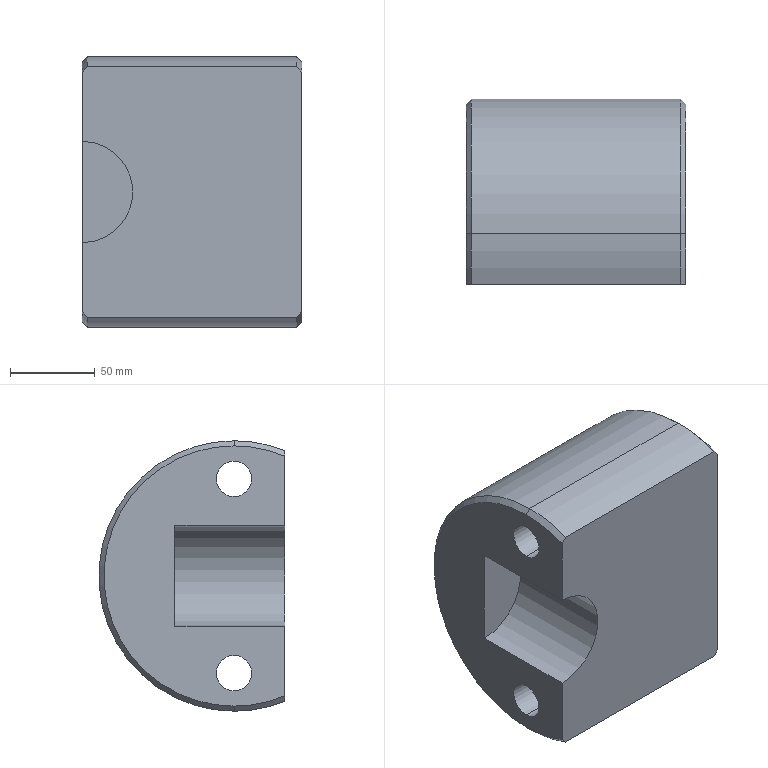Part | SolidWorks | features BaseBody 1 | 1 solid | 18 faces | box 130 x 110 x 160 mm | volume 1731219 mm3 | cylinder 8 | cone 6 | plane 4 | commonest cylinder face diameters 21 x4 160 x3 60 x1
STEP:
#1=CARTESIAN_POINT('',(240.077,193.635,-171.893));
#2=VERTEX_POINT('',#1);
#3=CARTESIAN_POINT('',(370.077,193.635,-171.893));
#4=VERTEX_POINT('',#3);
#5=CARTESIAN_POINT('',(370.077,193.635,-171.893));
#6=DIRECTION('',(1.,0.,0.));
#7=VECTOR('',#6,1000.);
#8=LINE('',#5,#7);
#9=EDGE_CURVE('',#2,#4,#8,.T.);
#10=ORIENTED_EDGE('',*,*,#9,.F.);
#11=CARTESIAN_POINT('',(240.077,193.635,-192.893));
#12=VERTEX_POINT('',#11);
#13=CARTESIAN_POINT('',(240.077,193.635,-182.393));
#14=DIRECTION('',(1.,0.,0.));
#15=DIRECTION('',(0.,0.,-1.));
#16=AXIS2_PLACEMENT_3D('',#13,#14,#15);
#17=CIRCLE('',#16,10.5);
#18=EDGE_CURVE('',#12,#2,#17,.T.);
#19=ORIENTED_EDGE('',*,*,#18,.F.);
#20=CARTESIAN_POINT('',(370.077,193.635,-192.893));
#21=VERTEX_POINT('',#20);
#22=CARTESIAN_POINT('',(370.077,193.635,-192.893));
#23=DIRECTION('',(1.,0.,0.));
#24=VECTOR('',#23,1000.);
#25=LINE('',#22,#24);
#26=EDGE_CURVE('',#12,#21,#25,.T.);
#27=ORIENTED_EDGE('',*,*,#26,.T.);
#28=CARTESIAN_POINT('',(370.077,193.635,-182.393));
#29=DIRECTION('',(1.,0.,0.));
#30=DIRECTION('',(0.,0.,-1.));
#31=AXIS2_PLACEMENT_3D('',#28,#29,#30);
#32=CIRCLE('',#31,10.5);
#33=EDGE_CURVE('',#21,#4,#32,.T.);
#34=ORIENTED_EDGE('',*,*,#33,.T.);
#35=EDGE_LOOP('',(#10,#19,#27,#34));
#36=FACE_OUTER_BOUND('',#35,.T.);
#37=CARTESIAN_POINT('',(370.077,193.635,-182.393));
#38=DIRECTION('',(1.,0.,0.));
#39=DIRECTION('',(0.,0.,-1.));
#40=AXIS2_PLACEMENT_3D('',#37,#38,#39);
#41=CYLINDRICAL_SURFACE('',#40,10.5);
#42=ADVANCED_FACE('',(#36),#41,.F.);
#43=CARTESIAN_POINT('',(240.077,193.635,-286.893));
#44=VERTEX_POINT('',#43);
#45=CARTESIAN_POINT('',(370.077,193.635,-286.893));
#46=VERTEX_POINT('',#45);
#47=CARTESIAN_POINT('',(370.077,193.635,-286.893));
#48=DIRECTION('',(1.,0.,0.));
#49=VECTOR('',#48,1000.);
#50=LINE('',#47,#49);
#51=EDGE_CURVE('',#44,#46,#50,.T.);
#52=ORIENTED_EDGE('',*,*,#51,.F.);
#53=CARTESIAN_POINT('',(240.077,193.635,-307.893));
#54=VERTEX_POINT('',#53);
#55=CARTESIAN_POINT('',(240.077,193.635,-297.393));
#56=DIRECTION('',(1.,0.,0.));
#57=DIRECTION('',(0.,0.,-1.));
#58=AXIS2_PLACEMENT_3D('',#55,#56,#57);
#59=CIRCLE('',#58,10.5);
#60=EDGE_CURVE('',#54,#44,#59,.T.);
#61=ORIENTED_EDGE('',*,*,#60,.F.);
#62=CARTESIAN_POINT('',(370.077,193.635,-307.893));
#63=VERTEX_POINT('',#62);
#64=CARTESIAN_POINT('',(370.077,193.635,-307.893));
#65=DIRECTION('',(1.,0.,0.));
#66=VECTOR('',#65,1000.);
#67=LINE('',#64,#66);
#68=EDGE_CURVE('',#54,#63,#67,.T.);
#69=ORIENTED_EDGE('',*,*,#68,.T.);
#70=CARTESIAN_POINT('',(370.077,193.635,-297.393));
#71=DIRECTION('',(1.,0.,0.));
#72=DIRECTION('',(0.,0.,-1.));
#73=AXIS2_PLACEMENT_3D('',#70,#71,#72);
#74=CIRCLE('',#73,10.5);
#75=EDGE_CURVE('',#63,#46,#74,.T.);
#76=ORIENTED_EDGE('',*,*,#75,.T.);
#77=EDGE_LOOP('',(#52,#61,#69,#76));
#78=FACE_OUTER_BOUND('',#77,.T.);
#79=CARTESIAN_POINT('',(370.077,193.635,-297.393));
#80=DIRECTION('',(1.,0.,0.));
#81=DIRECTION('',(0.,0.,-1.));
#82=AXIS2_PLACEMENT_3D('',#79,#80,#81);
#83=CYLINDRICAL_SURFACE('',#82,10.5);
#84=ADVANCED_FACE('',(#78),#83,.F.);
#85=CARTESIAN_POINT('',(240.077,228.635,-269.893));
#86=VERTEX_POINT('',#85);
#87=CARTESIAN_POINT('',(240.077,228.635,-209.893));
#88=VERTEX_POINT('',#87);
#89=CARTESIAN_POINT('',(240.077,228.635,-239.893));
#90=DIRECTION('',(0.,-1.,0.));
#91=DIRECTION('',(0.,0.,-1.));
#92=AXIS2_PLACEMENT_3D('',#89,#90,#91);
#93=CIRCLE('',#92,30.);
#94=EDGE_CURVE('',#86,#88,#93,.T.);
#95=ORIENTED_EDGE('',*,*,#94,.F.);
#96=CARTESIAN_POINT('',(240.077,163.635,-269.893));
#97=VERTEX_POINT('',#96);
#98=CARTESIAN_POINT('',(240.077,228.635,-269.893));
#99=DIRECTION('',(0.,1.,0.));
#100=VECTOR('',#99,1000.);
#101=LINE('',#98,#100);
#102=EDGE_CURVE('',#97,#86,#101,.T.);
#103=ORIENTED_EDGE('',*,*,#102,.F.);
#104=CARTESIAN_POINT('',(240.077,163.635,-209.893));
#105=VERTEX_POINT('',#104);
#106=CARTESIAN_POINT('',(240.077,163.635,-239.893));
#107=DIRECTION('',(0.,-1.,0.));
#108=DIRECTION('',(0.,0.,-1.));
#109=AXIS2_PLACEMENT_3D('',#106,#107,#108);
#110=CIRCLE('',#109,30.);
#111=EDGE_CURVE('',#97,#105,#110,.T.);
#112=ORIENTED_EDGE('',*,*,#111,.T.);
#113=CARTESIAN_POINT('',(240.077,228.635,-209.893));
#114=DIRECTION('',(0.,-1.,0.));
#115=VECTOR('',#114,1000.);
#116=LINE('',#113,#115);
#117=EDGE_CURVE('',#88,#105,#116,.T.);
#118=ORIENTED_EDGE('',*,*,#117,.F.);
#119=EDGE_LOOP('',(#95,#103,#112,#118));
#120=FACE_OUTER_BOUND('',#119,.T.);
#121=CARTESIAN_POINT('',(240.077,228.635,-239.893));
#122=DIRECTION('',(0.,-1.,0.));
#123=DIRECTION('',(0.,0.,1.));
#124=AXIS2_PLACEMENT_3D('',#121,#122,#123);
#125=CYLINDRICAL_SURFACE('',#124,30.);
#126=ADVANCED_FACE('',(#120),#125,.F.);
#127=CARTESIAN_POINT('',(240.077,228.635,-239.893));
#128=DIRECTION('',(0.,0.,-1.));
#129=VECTOR('',#128,1000.);
#130=LINE('',#127,#129);
#131=EDGE_CURVE('',#88,#86,#130,.T.);
#132=ORIENTED_EDGE('',*,*,#131,.T.);
#133=ORIENTED_EDGE('',*,*,#94,.T.);
#134=EDGE_LOOP('',(#132,#133));
#135=FACE_OUTER_BOUND('',#134,.T.);
#136=CARTESIAN_POINT('',(240.077,228.635,-239.893));
#137=DIRECTION('',(0.,-1.,0.));
#138=DIRECTION('',(0.,0.,-1.));
#139=AXIS2_PLACEMENT_3D('',#136,#137,#138);
#140=PLANE('',#139);
#141=ADVANCED_FACE('',(#135),#140,.T.);
#142=CARTESIAN_POINT('',(240.077,193.635,-162.893));
#143=VERTEX_POINT('',#142);
#144=CARTESIAN_POINT('',(243.077,193.635,-159.893));
#145=VERTEX_POINT('',#144);
#146=CARTESIAN_POINT('',(243.077,193.635,-159.893));
#147=DIRECTION('',(0.7071,0.,0.7071));
#148=VECTOR('',#147,1000.);
#149=LINE('',#146,#148);
#150=EDGE_CURVE('',#143,#145,#149,.T.);
#151=ORIENTED_EDGE('',*,*,#150,.F.);
#152=CARTESIAN_POINT('',(240.077,163.635,-168.978));
#153=VERTEX_POINT('',#152);
#154=CARTESIAN_POINT('',(240.077,193.635,-239.893));
#155=DIRECTION('',(-1.,0.,0.));
#156=DIRECTION('',(0.,0.,-1.));
#157=AXIS2_PLACEMENT_3D('',#154,#155,#156);
#158=CIRCLE('',#157,77.);
#159=EDGE_CURVE('',#153,#143,#158,.T.);
#160=ORIENTED_EDGE('',*,*,#159,.F.);
#161=CARTESIAN_POINT('',(243.077,163.635,-165.731));
#162=VERTEX_POINT('',#161);
#163=CARTESIAN_POINT('',(243.077,163.635,-165.731));
#164=CARTESIAN_POINT('',(242.075,163.635,-166.812));
#165=CARTESIAN_POINT('',(241.075,163.635,-167.894));
#166=CARTESIAN_POINT('',(240.077,163.635,-168.978));
#167=B_SPLINE_CURVE_WITH_KNOTS('',3,(#163,#164,#165,#166),.UNSPECIFIED.,.F.,.F.,(4,4),(0.,1.),.UNSPECIFIED.);
#168=EDGE_CURVE('',#162,#153,#167,.T.);
#169=ORIENTED_EDGE('',*,*,#168,.F.);
#170=CARTESIAN_POINT('',(243.077,193.635,-239.893));
#171=DIRECTION('',(1.,0.,0.));
#172=DIRECTION('',(0.,0.,-1.));
#173=AXIS2_PLACEMENT_3D('',#170,#171,#172);
#174=CIRCLE('',#173,80.);
#175=EDGE_CURVE('',#145,#162,#174,.T.);
#176=ORIENTED_EDGE('',*,*,#175,.F.);
#177=EDGE_LOOP('',(#151,#160,#169,#176));
#178=FACE_OUTER_BOUND('',#177,.T.);
#179=CARTESIAN_POINT('',(243.077,193.635,-239.893));
#180=DIRECTION('',(1.,0.,0.));
#181=DIRECTION('',(0.,0.,1.));
#182=AXIS2_PLACEMENT_3D('',#179,#180,#181);
#183=CONICAL_SURFACE('',#182,80.,0.7854);
#184=ADVANCED_FACE('',(#178),#183,.T.);
#185=CARTESIAN_POINT('',(370.077,193.635,-316.893));
#186=VERTEX_POINT('',#185);
#187=CARTESIAN_POINT('',(367.077,193.635,-319.893));
#188=VERTEX_POINT('',#187);
#189=CARTESIAN_POINT('',(370.077,193.635,-316.893));
#190=DIRECTION('',(-0.7071,0.,-0.7071));
#191=VECTOR('',#190,1000.);
#192=LINE('',#189,#191);
#193=EDGE_CURVE('',#186,#188,#192,.T.);
#194=ORIENTED_EDGE('',*,*,#193,.F.);
#195=CARTESIAN_POINT('',(370.077,163.635,-310.809));
#196=VERTEX_POINT('',#195);
#197=CARTESIAN_POINT('',(370.077,193.635,-239.893));
#198=DIRECTION('',(1.,0.,0.));
#199=DIRECTION('',(0.,0.,-1.));
#200=AXIS2_PLACEMENT_3D('',#197,#198,#199);
#201=CIRCLE('',#200,77.);
#202=EDGE_CURVE('',#196,#186,#201,.T.);
#203=ORIENTED_EDGE('',*,*,#202,.F.);
#204=CARTESIAN_POINT('',(367.077,163.635,-314.055));
#205=VERTEX_POINT('',#204);
#206=CARTESIAN_POINT('',(367.077,163.635,-314.055));
#207=CARTESIAN_POINT('',(368.079,163.635,-312.975));
#208=CARTESIAN_POINT('',(369.079,163.635,-311.893));
#209=CARTESIAN_POINT('',(370.077,163.635,-310.809));
#210=B_SPLINE_CURVE_WITH_KNOTS('',3,(#206,#207,#208,#209),.UNSPECIFIED.,.F.,.F.,(4,4),(0.,1.),.UNSPECIFIED.);
#211=EDGE_CURVE('',#205,#196,#210,.T.);
#212=ORIENTED_EDGE('',*,*,#211,.F.);
#213=CARTESIAN_POINT('',(367.077,193.635,-239.893));
#214=DIRECTION('',(-1.,0.,0.));
#215=DIRECTION('',(0.,0.,-1.));
#216=AXIS2_PLACEMENT_3D('',#213,#214,#215);
#217=CIRCLE('',#216,80.);
#218=EDGE_CURVE('',#188,#205,#217,.T.);
#219=ORIENTED_EDGE('',*,*,#218,.F.);
#220=EDGE_LOOP('',(#194,#203,#212,#219));
#221=FACE_OUTER_BOUND('',#220,.T.);
#222=CARTESIAN_POINT('',(370.077,193.635,-239.893));
#223=DIRECTION('',(-1.,0.,0.));
#224=DIRECTION('',(0.,0.,-1.));
#225=AXIS2_PLACEMENT_3D('',#222,#223,#224);
#226=CONICAL_SURFACE('',#225,77.,0.7854);
#227=ADVANCED_FACE('',(#221),#226,.T.);
#228=CARTESIAN_POINT('',(240.077,163.635,-239.893));
#229=DIRECTION('',(0.,0.,-1.));
#230=VECTOR('',#229,1000.);
#231=LINE('',#228,#230);
#232=EDGE_CURVE('',#153,#105,#231,.T.);
#233=ORIENTED_EDGE('',*,*,#232,.T.);
#234=ORIENTED_EDGE('',*,*,#111,.F.);
#235=CARTESIAN_POINT('',(240.077,163.635,-310.809));
#236=VERTEX_POINT('',#235);
#237=CARTESIAN_POINT('',(240.077,163.635,-239.893));
#238=DIRECTION('',(0.,0.,-1.));
#239=VECTOR('',#238,1000.);
#240=LINE('',#237,#239);
#241=EDGE_CURVE('',#97,#236,#240,.T.);
#242=ORIENTED_EDGE('',*,*,#241,.T.);
#243=CARTESIAN_POINT('',(243.077,163.635,-314.055));
#244=VERTEX_POINT('',#243);
#245=CARTESIAN_POINT('',(240.077,163.635,-310.809));
#246=CARTESIAN_POINT('',(241.075,163.635,-311.893));
#247=CARTESIAN_POINT('',(242.075,163.635,-312.975));
#248=CARTESIAN_POINT('',(243.077,163.635,-314.055));
#249=B_SPLINE_CURVE_WITH_KNOTS('',3,(#245,#246,#247,#248),.UNSPECIFIED.,.F.,.F.,(4,4),(0.,1.),.UNSPECIFIED.);
#250=EDGE_CURVE('',#236,#244,#249,.T.);
#251=ORIENTED_EDGE('',*,*,#250,.T.);
#252=CARTESIAN_POINT('',(370.077,163.635,-314.055));
#253=DIRECTION('',(-1.,0.,0.));
#254=VECTOR('',#253,1000.);
#255=LINE('',#252,#254);
#256=EDGE_CURVE('',#205,#244,#255,.T.);
#257=ORIENTED_EDGE('',*,*,#256,.F.);
#258=ORIENTED_EDGE('',*,*,#211,.T.);
#259=CARTESIAN_POINT('',(370.077,163.635,-168.978));
#260=VERTEX_POINT('',#259);
#261=CARTESIAN_POINT('',(370.077,163.635,-239.893));
#262=DIRECTION('',(0.,0.,-1.));
#263=VECTOR('',#262,1000.);
#264=LINE('',#261,#263);
#265=EDGE_CURVE('',#260,#196,#264,.T.);
#266=ORIENTED_EDGE('',*,*,#265,.F.);
#267=CARTESIAN_POINT('',(367.077,163.635,-165.731));
#268=VERTEX_POINT('',#267);
#269=CARTESIAN_POINT('',(370.077,163.635,-168.978));
#270=CARTESIAN_POINT('',(369.079,163.635,-167.894));
#271=CARTESIAN_POINT('',(368.079,163.635,-166.812));
#272=CARTESIAN_POINT('',(367.077,163.635,-165.731));
#273=B_SPLINE_CURVE_WITH_KNOTS('',3,(#269,#270,#271,#272),.UNSPECIFIED.,.F.,.F.,(4,4),(0.,1.),.UNSPECIFIED.);
#274=EDGE_CURVE('',#260,#268,#273,.T.);
#275=ORIENTED_EDGE('',*,*,#274,.T.);
#276=CARTESIAN_POINT('',(370.077,163.635,-165.731));
#277=DIRECTION('',(-1.,0.,0.));
#278=VECTOR('',#277,1000.);
#279=LINE('',#276,#278);
#280=EDGE_CURVE('',#268,#162,#279,.T.);
#281=ORIENTED_EDGE('',*,*,#280,.T.);
#282=ORIENTED_EDGE('',*,*,#168,.T.);
#283=EDGE_LOOP('',(#233,#234,#242,#251,#257,#258,#266,#275,#281,#282));
#284=FACE_OUTER_BOUND('',#283,.T.);
#285=CARTESIAN_POINT('',(370.077,163.635,-239.893));
#286=DIRECTION('',(0.,1.,0.));
#287=DIRECTION('',(1.,0.,0.));
#288=AXIS2_PLACEMENT_3D('',#285,#286,#287);
#289=PLANE('',#288);
#290=ADVANCED_FACE('',(#284),#289,.F.);
#291=CARTESIAN_POINT('',(243.077,193.635,-319.893));
#292=VERTEX_POINT('',#291);
#293=CARTESIAN_POINT('',(370.077,193.635,-319.893));
#294=DIRECTION('',(-1.,0.,0.));
#295=VECTOR('',#294,1000.);
#296=LINE('',#293,#295);
#297=EDGE_CURVE('',#188,#292,#296,.T.);
#298=ORIENTED_EDGE('',*,*,#297,.F.);
#299=ORIENTED_EDGE('',*,*,#218,.T.);
#300=ORIENTED_EDGE('',*,*,#256,.T.);
#301=CARTESIAN_POINT('',(243.077,193.635,-239.893));
#302=DIRECTION('',(1.,0.,0.));
#303=DIRECTION('',(0.,0.,-1.));
#304=AXIS2_PLACEMENT_3D('',#301,#302,#303);
#305=CIRCLE('',#304,80.);
#306=EDGE_CURVE('',#244,#292,#305,.T.);
#307=ORIENTED_EDGE('',*,*,#306,.T.);
#308=EDGE_LOOP('',(#298,#299,#300,#307));
#309=FACE_OUTER_BOUND('',#308,.T.);
#310=CARTESIAN_POINT('',(370.077,193.635,-239.893));
#311=DIRECTION('',(-1.,0.,0.));
#312=DIRECTION('',(0.,0.,-1.));
#313=AXIS2_PLACEMENT_3D('',#310,#311,#312);
#314=CYLINDRICAL_SURFACE('',#313,80.);
#315=ADVANCED_FACE('',(#309),#314,.T.);
#316=ORIENTED_EDGE('',*,*,#60,.T.);
#317=CARTESIAN_POINT('',(240.077,193.635,-297.393));
#318=DIRECTION('',(1.,0.,0.));
#319=DIRECTION('',(0.,0.,-1.));
#320=AXIS2_PLACEMENT_3D('',#317,#318,#319);
#321=CIRCLE('',#320,10.5);
#322=EDGE_CURVE('',#44,#54,#321,.T.);
#323=ORIENTED_EDGE('',*,*,#322,.T.);
#324=EDGE_LOOP('',(#316,#323));
#325=FACE_BOUND('',#324,.T.);
#326=ORIENTED_EDGE('',*,*,#18,.T.);
#327=CARTESIAN_POINT('',(240.077,193.635,-182.393));
#328=DIRECTION('',(1.,0.,0.));
#329=DIRECTION('',(0.,0.,-1.));
#330=AXIS2_PLACEMENT_3D('',#327,#328,#329);
#331=CIRCLE('',#330,10.5);
#332=EDGE_CURVE('',#2,#12,#331,.T.);
#333=ORIENTED_EDGE('',*,*,#332,.T.);
#334=EDGE_LOOP('',(#326,#333));
#335=FACE_BOUND('',#334,.T.);
#336=ORIENTED_EDGE('',*,*,#131,.F.);
#337=ORIENTED_EDGE('',*,*,#117,.T.);
#338=ORIENTED_EDGE('',*,*,#232,.F.);
#339=ORIENTED_EDGE('',*,*,#159,.T.);
#340=CARTESIAN_POINT('',(240.077,193.635,-316.893));
#341=VERTEX_POINT('',#340);
#342=CARTESIAN_POINT('',(240.077,193.635,-239.893));
#343=DIRECTION('',(-1.,0.,0.));
#344=DIRECTION('',(0.,0.,-1.));
#345=AXIS2_PLACEMENT_3D('',#342,#343,#344);
#346=CIRCLE('',#345,77.);
#347=EDGE_CURVE('',#143,#341,#346,.T.);
#348=ORIENTED_EDGE('',*,*,#347,.T.);
#349=CARTESIAN_POINT('',(240.077,193.635,-239.893));
#350=DIRECTION('',(-1.,0.,0.));
#351=DIRECTION('',(0.,0.,-1.));
#352=AXIS2_PLACEMENT_3D('',#349,#350,#351);
#353=CIRCLE('',#352,77.);
#354=EDGE_CURVE('',#341,#236,#353,.T.);
#355=ORIENTED_EDGE('',*,*,#354,.T.);
#356=ORIENTED_EDGE('',*,*,#241,.F.);
#357=ORIENTED_EDGE('',*,*,#102,.T.);
#358=EDGE_LOOP('',(#336,#337,#338,#339,#348,#355,#356,#357));
#359=FACE_OUTER_BOUND('',#358,.T.);
#360=CARTESIAN_POINT('',(240.077,193.635,-239.893));
#361=DIRECTION('',(1.,0.,0.));
#362=DIRECTION('',(0.,1.,0.));
#363=AXIS2_PLACEMENT_3D('',#360,#361,#362);
#364=PLANE('',#363);
#365=ADVANCED_FACE('',(#325,#335,#359),#364,.F.);
#366=ORIENTED_EDGE('',*,*,#75,.F.);
#367=CARTESIAN_POINT('',(370.077,193.635,-297.393));
#368=DIRECTION('',(1.,0.,0.));
#369=DIRECTION('',(0.,0.,-1.));
#370=AXIS2_PLACEMENT_3D('',#367,#368,#369);
#371=CIRCLE('',#370,10.5);
#372=EDGE_CURVE('',#46,#63,#371,.T.);
#373=ORIENTED_EDGE('',*,*,#372,.F.);
#374=EDGE_LOOP('',(#366,#373));
#375=FACE_BOUND('',#374,.T.);
#376=ORIENTED_EDGE('',*,*,#33,.F.);
#377=CARTESIAN_POINT('',(370.077,193.635,-182.393));
#378=DIRECTION('',(1.,0.,0.));
#379=DIRECTION('',(0.,0.,-1.));
#380=AXIS2_PLACEMENT_3D('',#377,#378,#379);
#381=CIRCLE('',#380,10.5);
#382=EDGE_CURVE('',#4,#21,#381,.T.);
#383=ORIENTED_EDGE('',*,*,#382,.F.);
#384=EDGE_LOOP('',(#376,#383));
#385=FACE_BOUND('',#384,.T.);
#386=ORIENTED_EDGE('',*,*,#265,.T.);
#387=ORIENTED_EDGE('',*,*,#202,.T.);
#388=CARTESIAN_POINT('',(370.077,193.635,-162.893));
#389=VERTEX_POINT('',#388);
#390=CARTESIAN_POINT('',(370.077,193.635,-239.893));
#391=DIRECTION('',(1.,0.,0.));
#392=DIRECTION('',(0.,0.,-1.));
#393=AXIS2_PLACEMENT_3D('',#390,#391,#392);
#394=CIRCLE('',#393,77.);
#395=EDGE_CURVE('',#186,#389,#394,.T.);
#396=ORIENTED_EDGE('',*,*,#395,.T.);
#397=CARTESIAN_POINT('',(370.077,193.635,-239.893));
#398=DIRECTION('',(1.,0.,0.));
#399=DIRECTION('',(0.,0.,-1.));
#400=AXIS2_PLACEMENT_3D('',#397,#398,#399);
#401=CIRCLE('',#400,77.);
#402=EDGE_CURVE('',#389,#260,#401,.T.);
#403=ORIENTED_EDGE('',*,*,#402,.T.);
#404=EDGE_LOOP('',(#386,#387,#396,#403));
#405=FACE_OUTER_BOUND('',#404,.T.);
#406=CARTESIAN_POINT('',(370.077,193.635,-239.893));
#407=DIRECTION('',(1.,0.,0.));
#408=DIRECTION('',(0.,1.,0.));
#409=AXIS2_PLACEMENT_3D('',#406,#407,#408);
#410=PLANE('',#409);
#411=ADVANCED_FACE('',(#375,#385,#405),#410,.T.);
#412=CARTESIAN_POINT('',(367.077,193.635,-159.893));
#413=VERTEX_POINT('',#412);
#414=CARTESIAN_POINT('',(367.077,193.635,-239.893));
#415=DIRECTION('',(-1.,0.,0.));
#416=DIRECTION('',(0.,0.,-1.));
#417=AXIS2_PLACEMENT_3D('',#414,#415,#416);
#418=CIRCLE('',#417,80.);
#419=EDGE_CURVE('',#268,#413,#418,.T.);
#420=ORIENTED_EDGE('',*,*,#419,.T.);
#421=CARTESIAN_POINT('',(370.077,193.635,-159.893));
#422=DIRECTION('',(-1.,0.,0.));
#423=VECTOR('',#422,1000.);
#424=LINE('',#421,#423);
#425=EDGE_CURVE('',#413,#145,#424,.T.);
#426=ORIENTED_EDGE('',*,*,#425,.T.);
#427=ORIENTED_EDGE('',*,*,#175,.T.);
#428=ORIENTED_EDGE('',*,*,#280,.F.);
#429=EDGE_LOOP('',(#420,#426,#427,#428));
#430=FACE_OUTER_BOUND('',#429,.T.);
#431=CARTESIAN_POINT('',(370.077,193.635,-239.893));
#432=DIRECTION('',(-1.,0.,0.));
#433=DIRECTION('',(0.,0.,-1.));
#434=AXIS2_PLACEMENT_3D('',#431,#432,#433);
#435=CYLINDRICAL_SURFACE('',#434,80.);
#436=ADVANCED_FACE('',(#430),#435,.T.);
#437=CARTESIAN_POINT('',(367.077,193.635,-239.893));
#438=DIRECTION('',(-1.,0.,0.));
#439=DIRECTION('',(0.,0.,-1.));
#440=AXIS2_PLACEMENT_3D('',#437,#438,#439);
#441=CIRCLE('',#440,80.);
#442=EDGE_CURVE('',#413,#188,#441,.T.);
#443=ORIENTED_EDGE('',*,*,#442,.T.);
#444=ORIENTED_EDGE('',*,*,#297,.T.);
#445=CARTESIAN_POINT('',(243.077,193.635,-239.893));
#446=DIRECTION('',(1.,0.,0.));
#447=DIRECTION('',(0.,0.,-1.));
#448=AXIS2_PLACEMENT_3D('',#445,#446,#447);
#449=CIRCLE('',#448,80.);
#450=EDGE_CURVE('',#292,#145,#449,.T.);
#451=ORIENTED_EDGE('',*,*,#450,.T.);
#452=ORIENTED_EDGE('',*,*,#425,.F.);
#453=EDGE_LOOP('',(#443,#444,#451,#452));
#454=FACE_OUTER_BOUND('',#453,.T.);
#455=CARTESIAN_POINT('',(370.077,193.635,-239.893));
#456=DIRECTION('',(-1.,0.,0.));
#457=DIRECTION('',(0.,0.,-1.));
#458=AXIS2_PLACEMENT_3D('',#455,#456,#457);
#459=CYLINDRICAL_SURFACE('',#458,80.);
#460=ADVANCED_FACE('',(#454),#459,.T.);
#461=ORIENTED_EDGE('',*,*,#402,.F.);
#462=CARTESIAN_POINT('',(370.077,193.635,-162.893));
#463=DIRECTION('',(-0.7071,0.,0.7071));
#464=VECTOR('',#463,1000.);
#465=LINE('',#462,#464);
#466=EDGE_CURVE('',#389,#413,#465,.T.);
#467=ORIENTED_EDGE('',*,*,#466,.T.);
#468=ORIENTED_EDGE('',*,*,#419,.F.);
#469=ORIENTED_EDGE('',*,*,#274,.F.);
#470=EDGE_LOOP('',(#461,#467,#468,#469));
#471=FACE_OUTER_BOUND('',#470,.T.);
#472=CARTESIAN_POINT('',(370.077,193.635,-239.893));
#473=DIRECTION('',(-1.,0.,0.));
#474=DIRECTION('',(0.,0.,-1.));
#475=AXIS2_PLACEMENT_3D('',#472,#473,#474);
#476=CONICAL_SURFACE('',#475,77.,0.7854);
#477=ADVANCED_FACE('',(#471),#476,.T.);
#478=ORIENTED_EDGE('',*,*,#395,.F.);
#479=ORIENTED_EDGE('',*,*,#193,.T.);
#480=ORIENTED_EDGE('',*,*,#442,.F.);
#481=ORIENTED_EDGE('',*,*,#466,.F.);
#482=EDGE_LOOP('',(#478,#479,#480,#481));
#483=FACE_OUTER_BOUND('',#482,.T.);
#484=CARTESIAN_POINT('',(370.077,193.635,-239.893));
#485=DIRECTION('',(-1.,0.,0.));
#486=DIRECTION('',(0.,0.,-1.));
#487=AXIS2_PLACEMENT_3D('',#484,#485,#486);
#488=CONICAL_SURFACE('',#487,77.,0.7854);
#489=ADVANCED_FACE('',(#483),#488,.T.);
#490=ORIENTED_EDGE('',*,*,#354,.F.);
#491=CARTESIAN_POINT('',(243.077,193.635,-319.893));
#492=DIRECTION('',(0.7071,0.,-0.7071));
#493=VECTOR('',#492,1000.);
#494=LINE('',#491,#493);
#495=EDGE_CURVE('',#341,#292,#494,.T.);
#496=ORIENTED_EDGE('',*,*,#495,.T.);
#497=ORIENTED_EDGE('',*,*,#306,.F.);
#498=ORIENTED_EDGE('',*,*,#250,.F.);
#499=EDGE_LOOP('',(#490,#496,#497,#498));
#500=FACE_OUTER_BOUND('',#499,.T.);
#501=CARTESIAN_POINT('',(243.077,193.635,-239.893));
#502=DIRECTION('',(1.,0.,0.));
#503=DIRECTION('',(0.,0.,1.));
#504=AXIS2_PLACEMENT_3D('',#501,#502,#503);
#505=CONICAL_SURFACE('',#504,80.,0.7854);
#506=ADVANCED_FACE('',(#500),#505,.T.);
#507=ORIENTED_EDGE('',*,*,#347,.F.);
#508=ORIENTED_EDGE('',*,*,#150,.T.);
#509=ORIENTED_EDGE('',*,*,#450,.F.);
#510=ORIENTED_EDGE('',*,*,#495,.F.);
#511=EDGE_LOOP('',(#507,#508,#509,#510));
#512=FACE_OUTER_BOUND('',#511,.T.);
#513=CARTESIAN_POINT('',(243.077,193.635,-239.893));
#514=DIRECTION('',(1.,0.,0.));
#515=DIRECTION('',(0.,0.,1.));
#516=AXIS2_PLACEMENT_3D('',#513,#514,#515);
#517=CONICAL_SURFACE('',#516,80.,0.7854);
#518=ADVANCED_FACE('',(#512),#517,.T.);
#519=ORIENTED_EDGE('',*,*,#322,.F.);
#520=ORIENTED_EDGE('',*,*,#51,.T.);
#521=ORIENTED_EDGE('',*,*,#372,.T.);
#522=ORIENTED_EDGE('',*,*,#68,.F.);
#523=EDGE_LOOP('',(#519,#520,#521,#522));
#524=FACE_OUTER_BOUND('',#523,.T.);
#525=CARTESIAN_POINT('',(370.077,193.635,-297.393));
#526=DIRECTION('',(1.,0.,0.));
#527=DIRECTION('',(0.,0.,-1.));
#528=AXIS2_PLACEMENT_3D('',#525,#526,#527);
#529=CYLINDRICAL_SURFACE('',#528,10.5);
#530=ADVANCED_FACE('',(#524),#529,.F.);
#531=ORIENTED_EDGE('',*,*,#332,.F.);
#532=ORIENTED_EDGE('',*,*,#9,.T.);
#533=ORIENTED_EDGE('',*,*,#382,.T.);
#534=ORIENTED_EDGE('',*,*,#26,.F.);
#535=EDGE_LOOP('',(#531,#532,#533,#534));
#536=FACE_OUTER_BOUND('',#535,.T.);
#537=CARTESIAN_POINT('',(370.077,193.635,-182.393));
#538=DIRECTION('',(1.,0.,0.));
#539=DIRECTION('',(0.,0.,-1.));
#540=AXIS2_PLACEMENT_3D('',#537,#538,#539);
#541=CYLINDRICAL_SURFACE('',#540,10.5);
#542=ADVANCED_FACE('',(#536),#541,.F.);
#543=CLOSED_SHELL('',(#42,#84,#126,#141,#184,#227,#290,#315,#365,#411,#436,#460,#477,#489,#506,#518,#530,#542));
#544=MANIFOLD_SOLID_BREP('',#543);
#545=CARTESIAN_POINT('',(0.,0.,0.));
#546=DIRECTION('',(0.,0.,1.));
#547=DIRECTION('',(1.,0.,0.));
#548=AXIS2_PLACEMENT_3D('',#545,#546,#547);
#549=(LENGTH_UNIT()NAMED_UNIT(*)SI_UNIT(.MILLI.,.METRE.));
#550=UNCERTAINTY_MEASURE_WITH_UNIT(LENGTH_MEASURE(0.00001),#549,'','');
#551=(NAMED_UNIT(*)PLANE_ANGLE_UNIT()SI_UNIT($,.RADIAN.));
#552=(NAMED_UNIT(*)SI_UNIT($,.STERADIAN.)SOLID_ANGLE_UNIT());
#553=(GEOMETRIC_REPRESENTATION_CONTEXT(3)GLOBAL_UNCERTAINTY_ASSIGNED_CONTEXT((#550))GLOBAL_UNIT_ASSIGNED_CONTEXT((#549,#551,#552))REPRESENTATION_CONTEXT('',''));
#554=ADVANCED_BREP_SHAPE_REPRESENTATION('',(#544,#548),#553);